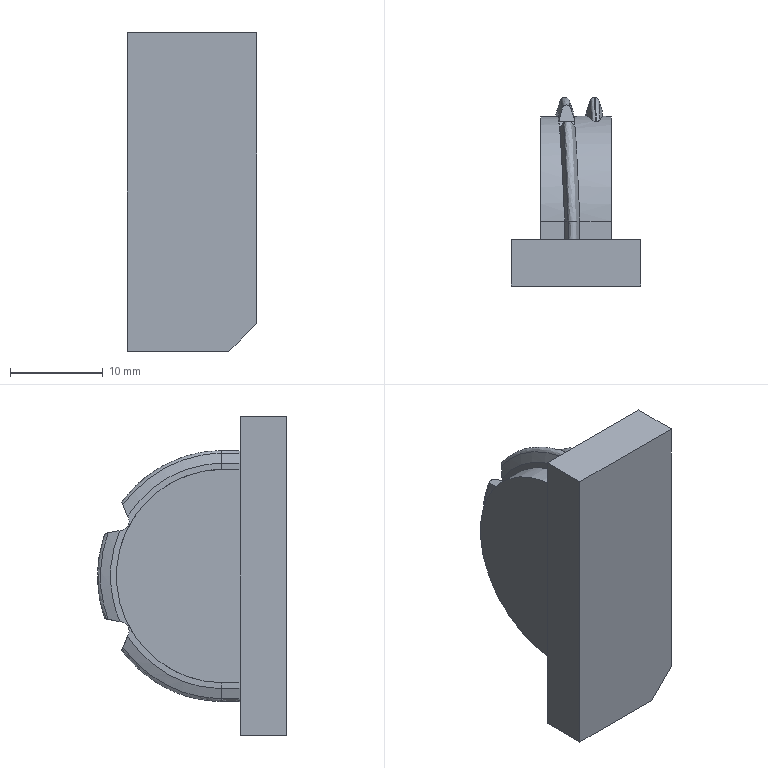NC program | NX | posted with a generic post | part box 13.933 x 20.347 x 34.335 mm
Lines 14732 to 15583 of 105565:
(ZLEVEL_PROFILE_1 , TOOL : B1)
N29432 M6
N29434 G54
N29436 G17 G0 G90 X-0.587 Y2.438 S3000 M3
N29438 G43 Z3. H0
N29440 Z0.049
N29442 G94 G1 X-0.056 Y2.545 Z0.035 F2000.
N29444 X-0.004 Y2.538 Z0.033
N29446 X0.121 Y2.496 Z0.03
N29448 X0.277 Y2.355 Z0.025
N29450 X0.373 Y2.168 Z0.019
N29452 X0.392 Y1.904 Z0.012
N29454 X0.323 Y1.706 Z0.007
N29456 X0.189 Y1.544 Z0.001
N29458 X0.071 Y1.484 Z-0.002
N29460 X-0.221 Y1.462 Z-0.01
N29462 X-0.784 Y1.533 Z-0.025
N29464 X-1.321 Y1.712 Z-0.04
N29466 X-1.575 Y1.858 Z-0.047
N29468 X-1.535 Y1.998 Z-0.051
N29470 X-1.39 Y2.186 Z-0.057
N29472 X-1.19 Y2.316 Z-0.064
N29474 X-0.056 Y2.545 Z-0.094
N29476 X-0.004 Y2.538 Z-0.095
N29478 X0.121 Y2.496 Z-0.099
N29480 X0.277 Y2.355 Z-0.104
N29482 X0.373 Y2.168 Z-0.11
N29484 X0.392 Y1.904 Z-0.117
N29486 X0.323 Y1.706 Z-0.122
N29488 X0.189 Y1.544 Z-0.128
N29490 X0.071 Y1.484 Z-0.131
N29492 X-0.221 Y1.462 Z-0.139
N29494 X-0.784 Y1.533 Z-0.154
N29496 X-1.321 Y1.712 Z-0.169
N29498 X-1.575 Y1.858 Z-0.176
N29500 X-1.535 Y1.998 Z-0.18
N29502 X-1.39 Y2.186 Z-0.186
N29504 X-1.19 Y2.316 Z-0.193
N29506 X-0.526 Y2.45 Z-0.21
N29508 X-0.056 Y2.545 F2500.
N29510 X-0.004 Y2.538
N29512 G2 X0.071 Y1.484 R0.574
N29514 X-1.575 Y1.858 R2.867
N29516 X-1.048 Y2.345 R0.692
N29518 G1 X-0.526 Y2.45
N29520 X-0.534 Y2.509 Z-0.24
N29522 X-0.543 Y2.566 Z-0.27
N29524 G3 X-1.957 Y2.124 R4.559
N29526 X-1.942 Y1.728 R0.218
N29528 X0.022 Y1.367 R4.774
N29530 X0.083 Y2.611 R0.661
N29532 X-0.543 Y2.566 R4.559
N29534 G1 X-0.548 Y2.604 Z-0.299
N29536 X-0.553 Y2.648 Z-0.329
N29538 G2 X-0.004 Y2.7 R7.638
N29540 X-0.004 Y1.296 R0.712
N29542 G1 X-0.176 Y1.301
N29544 G2 X-2.282 Y1.62 R7.678
N29546 X-2.304 Y2.204 R0.309
N29548 X-0.553 Y2.648 R7.638
N29550 G1 X-0.557 Y2.682 Z-0.358
N29552 X-0.561 Y2.718 Z-0.388
N29554 G3 X-2.608 Y2.252 R9.783
N29556 X-2.58 Y1.544 R0.37
N29558 X0.06 Y1.247 R9.406
N29560 X0.718 Y2.067 R0.847
N29562 X-0.004 Y2.767 R0.907
N29564 X-0.561 Y2.718 R9.783
N29566 G1 X-0.564 Y2.745 Z-0.418
N29568 X-0.566 Y2.775 Z-0.447
N29570 G2 X-0.349 Y2.792 R9.775
N29572 G1 X-0.176 Y2.81
N29574 G2 X0.341 Y2.684 R0.778
N29576 X0.824 Y1.895 R0.752
N29578 X-0.176 Y1.177 R1.03
N29580 X-2.879 Y1.504 R10.842
N29582 X-2.912 Y2.277 R0.404
N29584 X-0.566 Y2.775 R9.775
N29586 G1 X-0.568 Y2.798 Z-0.477
N29588 X-0.57 Y2.82 Z-0.507
N29590 G3 X-3.007 Y2.367 R12.019
N29592 X-3.462 Y1.819 R0.638
N29594 X-3.026 Y1.43 R0.647
N29596 X-1.222 Y1.164 R8.041
N29598 G1 X-0.176 Y1.13
N29600 G3 X0.749 Y1.55 R1.253
N29602 X0.685 Y2.532 R0.659
N29604 X-0.004 Y2.861 R1.736
N29606 G1 X-0.349 Y2.836
N29608 G3 X-0.57 Y2.82 R12.019
N29610 G1 X-0.572 Y2.844 Z-0.536
N29612 X-0.574 Y2.857 Z-0.566
N29614 X-0.214 Y2.893
N29616 G2 X0.341 Y2.795 R1.045
N29618 X0.856 Y2.471 R1.374
N29620 X0.848 Y1.545 R0.649
N29622 X-0.004 Y1.097 R1.725
N29624 X-2.972 Y1.295 R16.98
N29626 X-3.728 Y1.806 R1.071
N29628 X-3.3 Y2.362 R0.624
N29630 X-1.211 Y2.794 R9.295
N29632 G1 X-0.574 Y2.857
N29634 X-0.578 Y2.884 Z-0.596
N29636 X-0.58 Y2.901 Z-0.625
N29638 X-0.694 Y2.882
N29640 G3 X-2.8 Y2.588 R13.56
N29642 X-3.718 Y2.243 R3.437
N29644 X-3.682 Y1.457 R0.438
N29646 X-2.572 Y1.167 R3.663
N29648 X-0.004 Y1.065 R21.763
N29650 X0.954 Y1.55 R1.873
N29652 X0.85 Y2.584 R0.681
N29654 X-0.004 Y2.932 R2.125
N29656 X-0.58 Y2.901 R2.98
N29658 G1 X-0.582 Y2.919 Z-0.655
N29660 X-0.583 Y2.932 Z-0.685
N29662 G2 X-0.349 Y2.948 R22.545
N29664 X0.97 Y2.575 R1.894
N29666 X1.004 Y1.506 R0.686
N29668 X-0.004 Y1.034 R2.087
N29670 X-2.934 Y1.152 R21.479
N29672 X-3.957 Y1.503 R2.198
N29674 X-3.94 Y2.237 R0.432
N29676 X-2.769 Y2.666 R3.454
N29678 X-0.583 Y2.932 R22.545
N29680 G1 Y2.947 Z-0.714
N29682 X-0.584 Y2.958 Z-0.744
N29684 G3 X-2.934 Y2.685 R21.653
N29686 X-4.123 Y2.244 R3.067
N29688 X-4.059 Y1.406 R0.476
N29690 X-2.417 Y1.045 R4.349
N29692 X-0.176 Y1.009 R37.841
N29694 X1.101 Y1.505 R2.039
N29696 X1.048 Y2.6 R0.697
N29698 X0.168 Y2.955 R2.043
N29700 X-0.176 Y2.99 R2.299
N29702 G1 X-0.349 Y2.971
N29704 G3 X-0.584 Y2.958 R21.653
N29706 G1 X-0.585 Y2.972 Z-0.773
N29708 Y2.98 Z-0.803
N29710 G2 X-0.349 Y2.993 R26.082
N29712 G1 X-0.176 Y3.015
N29714 X-0.004 Y3.002
N29716 G2 X1.072 Y2.664 R2.478
N29718 X1.119 Y1.424 R0.738
N29720 X-0.262 Y0.989 R2.401
N29722 G1 X-0.521
N29724 X-1.498 Y0.987
N29726 G2 X-2.978 Y1.046 R17.456
N29728 X-4.276 Y1.408 R3.567
N29730 X-4.307 Y2.25 R0.48
N29732 X-2.934 Y2.734 R3.708
N29734 X-0.585 Y2.98 R26.082
N29736 G1 X-0.587 Y2.995 Z-0.833
N29738 Y3.001 Z-0.862
N29740 X-0.866 Y2.978
N29742 X-1.038 Y2.972
N29744 G3 X-3.107 Y2.747 R24.671
N29746 X-4.511 Y2.239 R3.589
N29748 X-4.428 Y1.378 R0.5
N29750 X-3.023 Y1.006 R3.791
N29752 X-1.494 Y0.961 R20.974
N29754 G1 X-0.521 Y0.968
N29756 X-0.28 Y0.969
N29758 G3 X1.21 Y1.42 R2.692
N29760 X1.291 Y2.562 R0.724
N29762 X0.685 Y2.892 R1.507
N29764 X-0.176 Y3.035 R3.755
N29766 G1 X-0.587 Y3.001
N29768 X-0.588 Y3.016 Z-0.892
N29770 X-0.589 Y3.027 Z-0.922
N29772 G2 X-0.176 Y3.054 R49.038
N29774 X0.654 Y2.932 R4.946
N29776 X1.324 Y2.624 R1.84
N29778 X1.286 Y1.409 R0.738
N29780 X-0.156 Y0.956 R2.857
N29782 X-2.934 Y0.968 R33.973
N29784 X-4.543 Y1.329 R4.34
N29786 X-4.59 Y2.304 R0.545
N29788 X-3.109 Y2.786 R4.049
N29790 X-0.589 Y3.027 R49.038
N29792 G1 X-0.59 Y3.036 Z-0.951
N29794 X-0.591 Y3.055 Z-0.981
N29796 G3 X-0.866 Y3.021 R3.751
N29798 X-3.452 Y2.762 R27.975
N29800 X-4.571 Y2.411 R4.36
N29802 X-4.49 Y1.206 R0.638
N29804 X-3.126 Y0.95 R5.191
N29806 X-1.162 Y0.916 R29.076
N29808 G1 X-0.521 Y0.926
N29810 X-0.364 Y0.927
N29812 G3 X0.965 Y1.187 R3.625
N29814 X1.488 Y1.516 R1.72
N29816 X1.474 Y2.584 R0.716
N29818 X0.685 Y2.958 R1.756
N29820 G1 X0.407 Y3.008
N29822 G3 X-0.591 Y3.055 R3.751
N29824 G1 X-0.592 Y3.068 Z-1.04
N29826 G2 X-0.176 Y3.093 R49.078
N29828 G1 X-0.004 Y3.076
N29830 X0.685 Y2.984
N29832 G2 X1.547 Y2.606 R1.843
N29834 X1.578 Y1.517 R0.722
N29836 X0.982 Y1.158 R1.731
N29838 X-0.176 Y0.908 R5.024
N29840 G1 X-0.521 Y0.905
N29842 X-0.694 Y0.902
N29844 G2 X-3.452 Y0.945 R32.317
N29846 X-4.831 Y1.293 R3.507
N29848 X-4.831 Y2.347 R0.783
N29850 X-3.452 Y2.796 R4.007
N29852 X-0.592 Y3.068 R49.078
N29854 G1 X-0.593 Y3.076 Z-1.07
N29856 Y3.086 Z-1.1
N29858 G3 X-3.279 Y2.844 R56.483
N29860 G1 X-3.624 Y2.799
N29862 G3 X-4.856 Y2.421 R4.211
N29864 X-5.069 Y1.722 R0.811
N29866 X-4.658 Y1.127 R0.575
N29868 X-3.279 Y0.901 R5.714
N29870 X-0.176 Y0.888 R53.64
N29872 X1.03 Y1.139 R6.428
N29874 X1.699 Y1.55 R1.73
N29876 X1.667 Y2.584 R0.726
N29878 X0.858 Y2.974 R1.713
N29880 G1 X0.685 Y3.008
N29882 X-0.176 Y3.112
N29884 G3 X-0.593 Y3.086 R56.483
N29886 G1 Z-0.9
N29888 G0 Z3.
N29890 X1.78 Y-0.901
N29892 Z0.049
N29894 G1 X1.815 Y-0.927 Z0.048 F2000.
N29896 X1.916 Y-1.082 Z0.043
N29898 X1.937 Y-1.206 Z0.04
N29900 X1.819 Y-1.344 Z0.035
N29902 X1.49 Y-1.534 Z0.025
N29904 X0.433 Y-1.734 Z-0.003
N29906 X-0.469 Y-1.764 Z-0.027
N29908 X-1.364 Y-1.649 Z-0.05
N29910 X-1.845 Y-1.509 Z-0.063
N29912 X-1.947 Y-1.38 Z-0.068
N29914 X-1.956 Y-1.198 Z-0.073
N29916 X-1.867 Y-1.06 Z-0.077
N29918 X-1.403 Y-0.876 Z-0.09
N29920 X-0.566 Y-0.682 Z-0.112
N29922 X0.291 Y-0.621 Z-0.135
N29924 X1.148 Y-0.692 Z-0.157
N29926 X1.667 Y-0.816 Z-0.171
N29928 X1.815 Y-0.927 Z-0.176
N29930 X1.916 Y-1.082 Z-0.181
N29932 X1.937 Y-1.206 Z-0.184
N29934 X1.819 Y-1.344 Z-0.189
N29936 X1.49 Y-1.534 Z-0.199
N29938 X1.073 Y-1.613 Z-0.21
N29940 X0.836 Y-1.658 F2500.
N29942 G2 X-1.758 Y-1.535 R5.585
N29944 X-1.782 Y-1.026 R0.269
N29946 X1.545 Y-0.786 R5.538
N29948 X1.937 Y-1.206 R0.521
N29950 X1.311 Y-1.568 R1.091
N29952 G1 X1.073 Y-1.613
N29954 X1.084 Y-1.673 Z-0.24
N29956 X1.094 Y-1.729 Z-0.27
N29958 G3 X1.589 Y-1.626 R7.56
N29960 X2.332 Y-1.206 R1.577
N29962 X1.999 Y-0.763 R0.434
N29964 X-2.091 Y-0.93 R7.483
N29966 X-2.067 Y-1.611 R0.355
N29968 X1.094 Y-1.729 R7.56
N29970 G1 X1.096 Y-1.773 Z-0.299
N29972 X1.098 Y-1.808 Z-0.329
N29974 X1.03 Y-1.811
N29976 G2 X-2.31 Y-1.689 R8.18
N29978 X-2.337 Y-0.882 R0.42
N29980 X1.691 Y-0.596 R8.496
N29982 G1 X2.236 Y-0.689
N29984 X2.503 Y-0.847
N29986 G2 X2.511 Y-1.366 R0.304
N29988 G1 X2.222 Y-1.55
N29990 X1.203 Y-1.803
N29992 X1.098 Y-1.808
N29994 X1.104 Y-1.85 Z-0.358
N29996 X1.107 Y-1.875 Z-0.388
N29998 G3 X2.45 Y-1.598 R11.001
N30000 X2.957 Y-1.033 R0.699
N30002 X2.416 Y-0.624 R0.816
N30004 X-0.004 Y-0.435 R8.638
N30006 X-2.634 Y-0.886 R7.722
N30008 X-2.969 Y-1.406 R0.506
N30010 X-2.173 Y-1.846 R1.338
N30012 X1.107 Y-1.875 R11.001
N30014 G1 X1.11 Y-1.91 Z-0.418
N30016 X1.111 Y-1.934 Z-0.447
N30018 X1.03 Y-1.94
N30020 X0.858 Y-1.958
N30022 G2 X-2.48 Y-1.875 R12.207
N30024 X-3.204 Y-1.444 R1.149
N30026 X-2.855 Y-0.861 R0.506
N30028 X-0.521 Y-0.407 R7.655
N30030 G1 X0.413 Y-0.374
N30032 G2 X2.064 Y-0.455 R9.732
N30034 G1 X2.904 Y-0.683
N30036 G2 X2.976 Y-1.454 R0.413
N30038 X1.203 Y-1.928 R4.786
N30040 G1 X1.111 Y-1.934
N30042 X1.113 Y-1.967 Z-0.477
N30044 Y-1.985 Z-0.507
N30046 G3 X3.202 Y-1.473 R5.552
N30048 X3.184 Y-0.685 R0.43
N30050 X1.922 Y-0.375 R4.363
N30052 X-0.377 Y-0.357 R13.847
N30054 G1 X-1.211 Y-0.419
N30056 G3 X-3.104 Y-0.861 R6.308
N30058 X-3.452 Y-1.45 R0.536
N30060 X-2.693 Y-1.906 R1.222
N30062 X1.03 Y-1.988 R12.577
N30064 G1 X1.113 Y-1.985
N30066 X1.116 Y-2.016 Z-0.536
N30068 X1.118 Y-2.033 Z-0.566
N30070 G2 X-2.073 Y-2.068 R18.508
N30072 X-3.446 Y-1.722 R3.773
N30074 X-3.476 Y-0.951 R0.431
N30076 X-2.146 Y-0.498 R4.116
N30078 X2.186 Y-0.344 R17.876
N30080 X3.446 Y-0.689 R3.552
N30082 X3.462 Y-1.453 R0.429
N30084 X2.068 Y-1.915 R4.32
N30086 X1.118 Y-2.033 R18.508
N30088 G1 X1.12 Y-2.054 Z-0.596
N30090 X1.121 Y-2.067 Z-0.625
N30092 G3 X2.237 Y-1.934 R21.035
N30094 X3.616 Y-1.496 R4.302
N30096 X3.616 Y-0.648 R0.465
N30098 X2.064 Y-0.283 R4.289
N30100 G1 X1.72 Y-0.26
N30102 G3 X-2.073 Y-0.437 R21.817
N30104 X-3.624 Y-0.902 R4.888
N30106 X-3.624 Y-1.766 R0.475
N30108 X-2.073 Y-2.121 R4.748
N30110 X1.121 Y-2.067 R21.035
N30112 G1 X1.123 Y-2.087 Z-0.655
N30114 X1.124 Y-2.1 Z-0.685
N30116 G2 X-2.245 Y-2.152 R25.232
N30118 X-3.907 Y-1.722 R3.995
N30120 X-3.763 Y-0.861 R0.52
N30122 X-2.417 Y-0.45 R4.296
N30124 X0.168 Y-0.23 R19.292
N30126 X2.983 Y-0.344 R14.916
N30128 X4.056 Y-0.861 R1.836
N30130 X3.805 Y-1.507 R0.514
N30132 X2.237 Y-1.983 R4.968
N30134 X1.124 Y-2.1 R25.232
N30136 G1 X1.125 Y-2.117 Z-0.714
N30138 X1.126 Y-2.127 Z-0.744
N30140 G3 X2.754 Y-1.936 R24.869
N30142 X4.133 Y-1.389 R3.285
N30144 X4.107 Y-0.689 R0.436
N30146 X3.099 Y-0.316 R2.297
N30148 G1 X2.582 Y-0.243
N30150 G3 X-0.176 Y-0.219 R19.973
N30152 X-2.762 Y-0.468 R18.319
N30154 X-4.07 Y-0.937 R3.537
N30156 X-4.044 Y-1.767 R0.476
N30158 X-2.59 Y-2.16 R3.554
N30160 X1.126 Y-2.127 R24.869
N30162 G1 X1.128 Y-2.144 Z-0.773
N30164 Y-2.153 Z-0.803
N30166 G2 X-2.66 Y-2.194 R28.227
N30168 X-4.141 Y-1.833 R4.196
N30170 G1 X-4.313 Y-1.729
N30172 G2 X-4.313 Y-0.995 R0.47
N30174 G1 X-4.134 Y-0.861
N30176 G2 X-2.59 Y-0.394 R4.542
N30178 X1.375 Y-0.162 R30.76
N30180 G1 X1.901 Y-0.17
N30182 G2 X3.423 Y-0.317 R9.243
N30184 X4.262 Y-0.653 R2.254
N30186 X4.24 Y-1.465 R0.478
N30188 X2.754 Y-1.979 R4.066
N30190 X1.128 Y-2.153 R28.227
N30192 G1 X1.129 Y-2.166 Z-0.833
N30194 X1.13 Y-2.174 Z-0.862
N30196 G3 X2.582 Y-2.034 R31.42
N30198 X4.127 Y-1.644 R5.955
N30200 X4.385 Y-1.512 R1.631
N30202 X4.303 Y-0.534 R0.552
N30204 X2.754 Y-0.178 R4.816
N30206 X-2.59 Y-0.364 R32.716
N30208 X-4.362 Y-0.883 R4.992
N30210 X-4.345 Y-1.839 R0.532
N30212 X-2.762 Y-2.217 R4.087
N30214 X1.13 Y-2.174 R31.42
N30216 G1 X1.131 Y-2.185 Z-0.892
N30218 Y-2.194 Z-0.922
N30220 G2 X-2.762 Y-2.248 R33.155
N30222 X-4.313 Y-1.958 R5.271
N30224 G1 X-4.54 Y-1.836
N30226 G2 X-4.542 Y-0.892 R0.537
N30228 G1 X-4.313 Y-0.768
N30230 G2 X-2.652 Y-0.344 R5.665
N30232 X2.926 Y-0.161 R34.752
N30234 X4.502 Y-0.543 R4.165
N30236 X4.541 Y-1.497 R0.537
N30238 X2.926 Y-2.015 R4.148
N30240 X1.131 Y-2.194 R33.155
N30242 G1 X1.132 Y-2.205 Z-0.951
N30244 X1.133 Y-2.213 Z-0.981
N30246 G3 X2.064 Y-2.133 R33.809
N30248 G1 X2.237 Y-2.117
N30250 X2.409 Y-2.109
N30252 G3 X3.616 Y-1.922 R11.817
N30254 X4.614 Y-1.55 R3.342
N30256 X4.626 Y-0.517 R0.59
N30258 G1 X4.478 Y-0.446
N30260 G3 X3.334 Y-0.169 R3.497
N30262 G1 X2.582 Y-0.118
N30264 X2.409 Y-0.119
N30266 X2.237 Y-0.113
N30268 G3 X-3.279 Y-0.407 R33.553
N30270 X-4.633 Y-0.854 R3.998
N30272 X-4.582 Y-1.916 R0.59
N30274 X-3.107 Y-2.254 R4.308
N30276 X1.133 Y-2.213 R33.809
N30278 G1 X1.134 Y-2.224 Z-1.011
N30280 Y-2.234 Z-1.04
N30282 G2 X-3.376 Y-2.263 R35.098
N30284 X-4.809 Y-1.895 R3.843
N30286 X-4.552 Y-0.714 R0.723
N30288 X-3.102 Y-0.353 R6.08
N30290 X2.926 Y-0.109 R37.765
N30292 X4.155 Y-0.267 R6.042
N30294 X4.813 Y-0.517 R2.655
N30296 X4.778 Y-1.55 R0.748
N30298 G1 X4.65 Y-1.626
N30300 X4.478 Y-1.705
N30302 X4.446 Y-1.722
N30304 G2 X2.966 Y-2.067 R6.616
N30306 G1 X2.108 Y-2.152
N30308 G2 X1.134 Y-2.234 R35.098
N30310 G1 X1.135 Y-2.244 Z-1.07
N30312 X1.136 Y-2.255 Z-1.1
N30314 G3 X2.926 Y-2.09 R37.837
N30316 G1 X3.117 Y-2.07
N30318 G3 X4.643 Y-1.708 R6.294
N30320 X5.045 Y-1.033 R0.628
N30322 X4.822 Y-0.435 R0.674
N30324 X4.133 Y-0.211 R2.583
N30326 X2.926 Y-0.084 R7.702
N30328 X-3.208 Y-0.344 R39.196
N30330 X-4.642 Y-0.689 R5.767
N30332 X-5.056 Y-1.378 R0.634
N30334 X-4.616 Y-2.067 R0.616
N30336 X-3.279 Y-2.296 R5.397
N30338 X1.136 Y-2.255 R37.837
N30340 G1 Y-2.263 Z-1.129
N30342 X1.137 Y-2.274 Z-1.159
N30344 G2 X-3.452 Y-2.312 R39.162
N30346 X-4.831 Y-2.046 R4.707
N30348 X-5.097 Y-1.378 R0.735
N30350 X-4.831 Y-0.712 R0.707
N30352 X-3.382 Y-0.344 R5.143
N30354 X3.435 Y-0.088 R39.169
N30356 X4.822 Y-0.352 R5.114
N30358 X5.085 Y-1.033 R0.759
N30360 X4.757 Y-1.722 R0.691
N30362 X3.314 Y-2.067 R6.305
N30364 X1.137 Y-2.274 R39.162
N30366 G1 Z-0.959
N30368 G0 Z3.
N30370 X0.411 Y0.949
N30372 Z-0.9
N30374 G1 X0.335 Y0.934 Z-0.902 F2000.
N30376 X-0.176 Y0.867 Z-0.915
N30378 X-1.464 Y0.836 Z-0.949
N30380 X-1.992 Y0.838 Z-0.963
N30382 X-3.279 Y0.878 Z-0.996
N30384 X-3.708 Y0.888 Z-1.008
N30386 X-4.243 Y0.962 Z-1.022
N30388 X-4.658 Y1.068 Z-1.033
N30390 X-4.785 Y1.096 Z-1.036
N30392 X-4.964 Y1.229 Z-1.042
N30394 X-5.077 Y1.421 Z-1.048
N30396 X-5.09 Y1.55 Z-1.051
N30398 X-5.115 Y1.805 Z-1.058
N30400 X-5.083 Y2.193 Z-1.068
N30402 X-4.983 Y2.382 Z-1.074
N30404 X-4.824 Y2.524 Z-1.08
N30406 X-4.299 Y2.703 Z-1.094
N30408 X-3.905 Y2.792 Z-1.105
N30410 X-2.667 Y2.938 Z-1.137
N30412 X-1.846 Y3.01 Z-1.159
N30414 G2 X-0.336 Y3.12 R54.456 F2500.
N30416 G1 X-0.176 Y3.13
N30418 X-0.004 Y3.112
N30420 X0.858 Y2.999
N30422 X1.03 Y2.96
N30424 G2 X1.76 Y2.584 R1.618
N30426 X1.784 Y1.55 R0.731
N30428 X1.03 Y1.11 R1.775
N30430 X-0.176 Y0.867 R8.852
N30432 X-3.279 Y0.878 R55.304
N30434 X-4.658 Y1.068 R6.129
N30436 X-5.09 Y1.55 R0.551
N30438 X-5.094 Y2.06 R2.87
N30440 X-4.698 Y2.567 R0.587
N30442 X-3.486 Y2.842 R5.919
N30444 X-1.846 Y3.01 R54.456
N30446 G1 X-1.847 Y3.021 Z-1.218
N30448 X-2.936 Y2.928
N30450 X-3.452 Y2.868
N30452 G3 X-4.767 Y2.594 R6.421
N30454 X-5.095 Y2.221 R0.484
N30456 X-5.09 Y1.415 R2.137
N30458 X-4.707 Y1.024 R0.499
N30460 X-3.279 Y0.856 R7.51
N30462 X-0.176 Y0.849 R56.44
N30464 G1 X-0.06 Y0.861
N30466 X0.827 Y1.033
N30468 X1.03 Y1.089
N30470 G3 X1.869 Y1.55 R1.775
N30472 X1.852 Y2.584 R0.737
N30474 X1.03 Y2.988 R1.702
N30476 G1 X0.858 Y3.021
N30478 X-0.176 Y3.148
N30480 X-0.694 Y3.12
N30482 X-1.847 Y3.021
N30484 Z-1.018
N30486 G0 Z3.
N30488 X1.438 Y-0.023
N30490 Z-0.959
N30492 G1 X2.355 Y-0.014 Z-0.983 F2000.
N30494 X3.443 Y-0.067 Z-1.011
N30496 X3.87 Y-0.082 Z-1.023
N30498 X4.235 Y-0.132 Z-1.032
N30500 X4.65 Y-0.232 Z-1.043
N30502 X4.777 Y-0.255 Z-1.047
N30504 X4.955 Y-0.379 Z-1.052
N30506 X5.072 Y-0.562 Z-1.058
N30508 X5.091 Y-0.689 Z-1.062
N30510 X5.127 Y-0.958 Z-1.069
N30512 Y-1.094 Z-1.072
N30514 X5.072 Y-1.486 Z-1.083
N30516 X4.879 Y-1.726 Z-1.091
N30518 X4.408 Y-1.901 Z-1.104
N30520 X4.161 Y-1.965 Z-1.11
N30522 X3.788 Y-2.019 Z-1.12
N30524 X2.723 Y-2.166 Z-1.148
N30526 X1.144 Y-2.308 Z-1.19
N30528 X0.069 Y-2.352 Z-1.218
N30530 G2 X-3.624 Y-2.325 R38.551 F2500.
N30532 X-4.658 Y-2.17 R6.592
N30534 X-5.099 Y-1.722 R0.544
N30536 X-5.097 Y-1.017 R2.094
N30538 X-4.776 Y-0.633 R0.501
N30540 X-3.547 Y-0.344 R5.227
N30542 X3.443 Y-0.067 R39.602
N30544 X4.65 Y-0.232 R6.065
N30546 X5.091 Y-0.689 R0.543
N30548 X5.089 Y-1.363 R2.452
N30550 X4.762 Y-1.77 R0.51
N30552 X3.788 Y-2.019 R4.735
N30554 X0.069 Y-2.352 R38.551
N30556 G1 X0.07 Y-2.362 Z-1.248
N30558 Y-2.372 Z-1.277
N30560 G3 X2.926 Y-2.148 R38.557
N30562 G1 X3.099 Y-2.129
N30564 G3 X4.659 Y-1.867 R11.419
N30566 X5.066 Y-1.55 R0.618
N30568 X5.092 Y-0.572 R1.929
N30570 X4.706 Y-0.195 R0.502
N30572 X3.616 Y-0.059 R6.789
N30574 X-3.107 Y-0.276 R38.2
N30576 G1 X-3.279 Y-0.291
N30578 G3 X-4.74 Y-0.562 R8.394
N30580 X-5.114 Y-0.966 R0.523
N30582 X-5.117 Y-1.78 R2.155
N30584 X-4.689 Y-2.212 R0.543
N30586 X-3.624 Y-2.346 R7.496
N30588 X0.07 Y-2.372 R38.557
N30590 G1 Z-1.077
N30592 G0 Z3.
N30594 X-2.829 Y2.958
N30596 Z-1.018
N30598 G1 X-2.161 Y3.032 Z-1.036 F2000.
N30600 X-0.866 Y3.127 Z-1.07
N30602 X-0.193 Y3.178 Z-1.087
N30604 X0.03 Y3.166 Z-1.093
N30606 X0.341 Y3.109 Z-1.102
N30608 X0.775 Y3.064 Z-1.113
N30610 X1.203 Y2.974 Z-1.124
N30612 X1.416 Y2.926 Z-1.13
N30614 X1.782 Y2.733 Z-1.141
N30616 X1.942 Y2.584 Z-1.147
N30618 X2.047 Y2.477 Z-1.151
N30620 X2.156 Y2.212 Z-1.158
N30622 X2.159 Y1.926 Z-1.166
N30624 X2.055 Y1.659 Z-1.173
N30626 X1.952 Y1.55 Z-1.177
N30628 X1.787 Y1.388 Z-1.183
N30630 X1.424 Y1.176 Z-1.194
N30632 X1.203 Y1.112 Z-1.2
N30634 X0.615 Y0.956 Z-1.216
N30636 X0.425 Y0.918 Z-1.221
N30638 X-0.176 Y0.831 Z-1.237
N30640 X-0.947 Y0.809 Z-1.257
N30642 X-1.717 Y0.811 Z-1.277
N30644 G2 X-3.279 Y0.836 R53.26 F2500.
N30646 X-4.658 Y0.969 R8.869
N30648 X-5.112 Y1.378 R0.529
N30650 X-5.121 Y2.225 R2.277
N30652 X-4.716 Y2.661 R0.551
N30654 X-3.452 Y2.889 R8.842
N30656 X-0.866 Y3.127 R70.143
N30658 G1 X-0.509 Y3.154
N30660 G2 X0.341 Y3.109 R3.322
N30662 X1.203 Y2.974 R8.424
N30664 X1.942 Y2.584 R1.592
N30666 X1.952 Y1.55 R0.743
N30668 X1.203 Y1.112 R1.771
N30670 X-0.176 Y0.831 R12.32
N30672 X-1.717 Y0.811 R53.26
N30674 G1 Y0.801 Z-1.307
N30676 Y0.788 Z-1.337
N30678 G3 X-0.176 Y0.812 R42.642
N30680 X1.203 Y1.092 R13.974
N30682 X2.034 Y1.55 R1.755
N30684 X1.892 Y2.706 R0.76
N30686 X1.203 Y3.001 R1.835
N30688 X-0.349 Y3.186 R10.767
N30690 G1 X-2.245 Y3.033
N30692 G3 X-4.482 Y2.756 R25.704
N30694 X-4.958 Y2.584 R1.2
N30696 X-5.169 Y2.048 R0.718
N30698 G1 X-5.17 Y1.967
N30700 Y1.609
N30702 X-5.169 Y1.594
N30704 X-5.158 Y1.453
N30706 G3 X-4.874 Y0.998 R0.584
N30708 X-4.12 Y0.861 R3.093
N30710 X-1.717 Y0.788 R42.642
N30712 G1 Z-1.137
N30714 G0 Z0.049
N30716 G1 X1.74 Y0.017 F5000.
N30718 G0 Z-1.077
N30720 G1 X2.892 Y0.01 Z-1.108 F2000.
N30722 X3.961 Y-0.059 Z-1.136
N30724 X4.65 Y-0.142 Z-1.154
N30726 X4.777 Y-0.154 Z-1.157
N30728 X4.941 Y-0.245 Z-1.162
N30730 X5.065 Y-0.387 Z-1.167
N30732 X5.159 Y-0.68 Z-1.175
N30734 Y-1.092 Z-1.186
N30736 X5.166 Y-1.298 Z-1.191
N30738 X5.159 Y-1.354 Z-1.193
N30740 X5.099 Y-1.55 Z-1.198
N30742 X5.055 Y-1.67 Z-1.201
N30744 X4.838 Y-1.86 Z-1.209
N30746 X4.099 Y-2.026 Z-1.229
N30748 X3.981 Y-2.046 Z-1.232
N30750 X3.099 Y-2.148 Z-1.255
N30752 X2.03 Y-2.277 Z-1.283
N30754 X1.074 Y-2.352 Z-1.309
N30756 X-0.002 Y-2.394 Z-1.337
N30758 G2 X-3.624 Y-2.366 R38.621 F2500.
N30760 X-4.74 Y-2.239 R7.862
N30762 X-5.114 Y-1.895 R0.502
N30764 X-5.17 Y-1.525 R1.297
N30766 G1 Y-1.32
N30768 G2 X-5.113 Y-0.861 R1.432
N30770 X-4.733 Y-0.517 R0.522
N30772 X-3.279 Y-0.273 R10.732
N30774 G1 X-3.107 Y-0.256
N30776 X-2.934 Y-0.236
N30778 G2 X3.961 Y-0.059 R38.189
N30780 G1 X4.65 Y-0.142
N30782 G2 X5.104 Y-0.508 R0.531
N30784 X5.159 Y-0.861 R1.155
N30786 G1 Y-1.092
N30788 G2 X5.099 Y-1.55 R1.402
N30790 X4.714 Y-1.888 R0.534
N30792 X3.356 Y-2.118 R13.217
N30794 G1 X3.099 Y-2.148
N30796 G2 X-0.002 Y-2.394 R38.621
N30798 G1 X-0.001 Y-2.404 Z-1.366
N30800 Y-2.415 Z-1.396
N30802 G3 X3.257 Y-2.148 R38.262
N30804 X4.675 Y-1.934 R28.803
N30806 X5.166 Y-1.378 R0.595
N30808 G1 X5.171 Y-1.283
N30810 Y-0.792
N30812 Y-0.779
N30814 X5.168 Y-0.689
N30816 G3 X4.822 Y-0.148 R0.611
N30818 X4.133 Y-0.048 R4.514
N30820 X-2.934 Y-0.217 R38.295
N30822 G1 X-3.107 Y-0.237
N30824 X-3.279 Y-0.254
N30826 G3 X-4.831 Y-0.508 R11.863
N30828 X-5.178 Y-1.033 R0.604
N30830 G1 X-5.182 Y-1.144
N30832 Y-1.654
N30834 G3 X-4.831 Y-2.253 R0.632
N30836 X-3.969 Y-2.363 R5.505
N30838 X-0.001 Y-2.415 R38.262
N30840 G1 Z-1.196
N30842 G0 Z3.
N30844 X-0.173 Y0.795
N30846 Z-1.137
N30848 G1 X-0.176 Y0.794 F2000.
N30850 X-1.326 Y0.755 Z-1.167
N30852 X-2.8 Y0.768 Z-1.206
N30854 X-4.382 Y0.85 Z-1.247
N30856 X-4.406 Y0.853 Z-1.248
N30858 X-4.831 Y0.937 Z-1.259
N30860 X-4.954 Y0.994 Z-1.263
N30862 X-5.108 Y1.167 Z-1.269
N30864 X-5.189 Y1.385 Z-1.275
N30866 X-5.182 Y1.52 Z-1.278
N30868 Y2.088 Z-1.293
N30870 X-5.166 Y2.347 Z-1.3
N30872 X-5.061 Y2.545 Z-1.306
N30874 X-4.887 Y2.686 Z-1.312
N30876 X-4.618 Y2.756 Z-1.319
N30878 X-3.703 Y2.909 Z-1.343
N30880 X-3.169 Y2.976 Z-1.357
N30882 X-2.245 Y3.052 Z-1.382
N30884 X-1.696 Y3.098 Z-1.396
N30886 X-0.694 Y3.182 F2500.
N30888 X-0.349 Y3.207
N30890 G2 X1.375 Y2.985 R12.635
N30892 X2.064 Y2.637 R1.611
N30894 X2.114 Y1.55 R0.756
N30896 X1.375 Y1.115 R1.747
N30898 X-0.176 Y0.794 R16.571
N30900 X-3.949 Y0.828 R44.109
N30902 X-4.831 Y0.937 R6.248
N30904 X-5.182 Y1.52 R0.609
N30906 G1 Y2.088
N30908 X-5.174 Y2.218
N30910 G2 X-4.762 Y2.719 R0.551
N30912 G1 X-4.618 Y2.756
N30914 G2 X-2.245 Y3.052 R28.661
N30916 G1 X-1.696 Y3.098
N30918 X-1.697 Y3.109 Z-1.426
N30920 X-1.698 Y3.117 Z-1.455
N30922 X-2.245 Y3.071
N30924 G3 X-4.711 Y2.762 R31.239
N30926 X-5.193 Y2.193 R0.577
N30928 G1 Y1.45
N30930 G3 X-4.653 Y0.865 R0.587
N30932 X-0.176 Y0.776 R37.333
N30934 G1 X-0.004 Y0.803
N30936 X1.203 Y1.051
N30938 X1.375 Y1.096
N30940 G3 X2.193 Y1.55 R1.738
N30942 X2.064 Y2.712 R0.77
N30944 X1.375 Y3.012 R1.851
N30946 X-0.349 Y3.227 R16.229
N30948 G1 X-0.694 Y3.202
N30950 X-1.698 Y3.117
N30952 Z-1.255
N30954 G0 Z3.
N30956 X3.962 Y-2.079
N30958 Z-1.196
N30960 G1 X3.658 Y-2.129 Z-1.204 F2000.
N30962 X1.245 Y-2.382 Z-1.268
N30964 X-1.179 Y-2.478 Z-1.331
N30966 X-3.604 Y-2.415 Z-1.395
N30968 X-4.658 Y-2.324 Z-1.422
N30970 X-4.79 Y-2.314 Z-1.426
N30972 X-5.061 Y-2.139 Z-1.434
N30974 X-5.2 Y-1.849 Z-1.443
N30976 X-5.193 Y-1.717 Z-1.446
N30978 Y-1.368 Z-1.455
N30980 Y-1.019 F2500.
N30982 G2 X-4.704 Y-0.442 R0.585
N30984 X4.478 Y-0.058 R37.792
N30986 X4.735 Y-0.094 R1.922
N30988 X5.182 Y-0.643 R0.561
N30990 G1 Y-1.388
N30992 G2 X4.701 Y-1.955 R0.575
N30994 X-4.658 Y-2.324 R37.31
N30996 X-5.193 Y-1.717 R0.579
N30998 G1 Y-1.368
N31000 X-5.205 Z-1.515
N31002 Y-1.761
N31004 G3 X-4.658 Y-2.35 R0.571
N31006 X4.712 Y-1.98 R38.302
N31008 X5.194 Y-1.413 R0.575
N31010 G1 Y-0.652
N31012 G3 X4.65 Y-0.049 R0.573
N31014 X-4.728 Y-0.424 R38.551
N31016 X-5.205 Y-0.986 R0.569
N31018 G1 Y-1.368
N31020 Z-1.315
N31022 G0 Z0.049
N31024 G1 X-0.429 Y0.748 F5000.
N31026 G0 Z-1.255
N31028 G1 X-1.223 Y0.714 Z-1.276 F2000.
N31030 X-3.614 Y0.761 Z-1.339
N31032 X-4.658 Y0.845 Z-1.366
N31034 X-4.79 Y0.85 Z-1.37
N31036 X-5.062 Y1.014 Z-1.378
N31038 X-5.208 Y1.297 Z-1.386
N31040 X-5.205 Y1.428 Z-1.39
N31042 Y2.356 Z-1.414
N31044 X-5.081 Y2.601 Z-1.421
N31046 X-4.858 Y2.761 Z-1.428
N31048 X-3.608 Y2.956 Z-1.462
N31050 X-2.722 Y3.06 Z-1.485
N31052 X-1.591 Y3.152 Z-1.515
N31054 G2 X-1.211 Y3.181 R42.901 F2500.
N31056 G1 X-0.349 Y3.248
N31058 G2 X1.547 Y2.993 R15.14
N31060 X2.24 Y2.63 R1.492
N31062 X2.241 Y1.522 R0.757
N31064 X1.456 Y1.096 R1.78
N31066 X-0.176 Y0.758 R21.423
N31068 X-4.658 Y0.845 R36.559
N31070 X-5.205 Y1.428 R0.568
N31072 G1 Y2.225
N31074 G2 X-4.729 Y2.781 R0.563
N31076 X-1.591 Y3.152 R42.901
N31078 G1 X-1.592 Y3.159 Z-1.544
N31080 X-1.593 Y3.173 Z-1.574
N31082 G3 X-4.734 Y2.803 R52.958
N31084 X-5.217 Y2.243 R0.566
N31086 G1 Y1.386
N31088 G3 X-4.703 Y0.828 R0.56
N31090 X-0.176 Y0.74 R36.112
N31092 G1 X-0.004 Y0.769
N31094 X1.284 Y1.033
N31096 X1.547 Y1.101
N31098 G3 X2.315 Y1.519 R1.721
N31100 X2.289 Y2.661 R0.769
N31102 X1.547 Y3.021 R1.608
N31104 X-0.349 Y3.268 R19.975
N31106 X-1.593 Y3.173 R52.958
N31108 G1 Z-1.374
N31110 G0 Z3.
N31112 X3.906 Y-2.131
N31114 Z-1.315
N31116 G1 X3.763 Y-2.155 Z-1.318 F2000.
N31118 X1.321 Y-2.414 Z-1.383
N31120 X-1.133 Y-2.516 Z-1.447
N31122 X-3.588 Y-2.462 Z-1.511
N31124 X-4.658 Y-2.374 Z-1.539
N31126 X-4.79 Y-2.371 Z-1.543
N31128 X-5.068 Y-2.209 Z-1.551